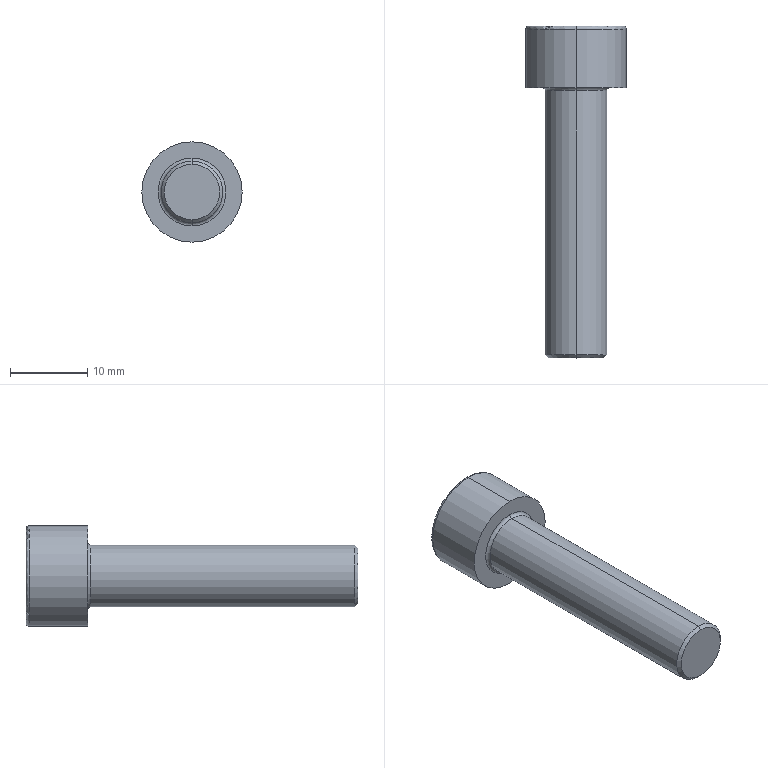Part | STEP file | 1 solid | 20 faces | box 13 x 43 x 13 mm | volume 2694 mm3 | plane 10 | torus 4 | cylinder 4 | cone 2 | commonest cylinder face diameters 8 x2 13 x2
STEP:
#1=CARTESIAN_POINT('',(0.,-35.,-3.6));
#2=VERTEX_POINT('',#1);
#3=CARTESIAN_POINT('',(0.,-35.,3.6));
#4=VERTEX_POINT('',#3);
#5=CARTESIAN_POINT('',(0.,-35.,0.));
#6=DIRECTION('',(0.,-1.,0.));
#7=DIRECTION('',(0.,0.,-1.));
#8=AXIS2_PLACEMENT_3D('',#5,#6,#7);
#9=CIRCLE('',#8,3.6);
#10=EDGE_CURVE('',#2,#4,#9,.T.);
#11=ORIENTED_EDGE('',*,*,#10,.F.);
#12=CARTESIAN_POINT('',(0.,-34.6,-4.));
#13=VERTEX_POINT('',#12);
#14=CARTESIAN_POINT('',(0.,-35.,-3.6));
#15=DIRECTION('',(0.,0.7071,-0.7071));
#16=VECTOR('',#15,1000.);
#17=LINE('',#14,#16);
#18=EDGE_CURVE('',#2,#13,#17,.T.);
#19=ORIENTED_EDGE('',*,*,#18,.T.);
#20=CARTESIAN_POINT('',(0.,-34.6,4.));
#21=VERTEX_POINT('',#20);
#22=CARTESIAN_POINT('',(0.,-34.6,0.));
#23=DIRECTION('',(0.,1.,0.));
#24=DIRECTION('',(0.,0.,-1.));
#25=AXIS2_PLACEMENT_3D('',#22,#23,#24);
#26=CIRCLE('',#25,4.);
#27=EDGE_CURVE('',#21,#13,#26,.T.);
#28=ORIENTED_EDGE('',*,*,#27,.F.);
#29=CARTESIAN_POINT('',(0.,-35.,3.6));
#30=DIRECTION('',(0.,0.7071,0.7071));
#31=VECTOR('',#30,1000.);
#32=LINE('',#29,#31);
#33=EDGE_CURVE('',#4,#21,#32,.T.);
#34=ORIENTED_EDGE('',*,*,#33,.F.);
#35=EDGE_LOOP('',(#11,#19,#28,#34));
#36=FACE_OUTER_BOUND('',#35,.T.);
#37=CARTESIAN_POINT('',(0.,-35.,0.));
#38=DIRECTION('',(0.,1.,0.));
#39=DIRECTION('',(0.,0.,1.));
#40=AXIS2_PLACEMENT_3D('',#37,#38,#39);
#41=CONICAL_SURFACE('',#40,3.6,0.7854);
#42=ADVANCED_FACE('',(#36),#41,.T.);
#43=CARTESIAN_POINT('',(0.,7.6,-6.5));
#44=VERTEX_POINT('',#43);
#45=CARTESIAN_POINT('',(0.,7.6,6.5));
#46=VERTEX_POINT('',#45);
#47=CARTESIAN_POINT('',(0.,7.6,0.));
#48=DIRECTION('',(0.,-1.,0.));
#49=DIRECTION('',(0.,0.,1.));
#50=AXIS2_PLACEMENT_3D('',#47,#48,#49);
#51=CIRCLE('',#50,6.5);
#52=EDGE_CURVE('',#44,#46,#51,.T.);
#53=ORIENTED_EDGE('',*,*,#52,.F.);
#54=CARTESIAN_POINT('',(0.,8.,-6.1));
#55=VERTEX_POINT('',#54);
#56=CARTESIAN_POINT('',(0.,7.6,-6.1));
#57=DIRECTION('',(1.,0.,0.));
#58=DIRECTION('',(0.,0.,-1.));
#59=AXIS2_PLACEMENT_3D('',#56,#57,#58);
#60=CIRCLE('',#59,0.4);
#61=EDGE_CURVE('',#44,#55,#60,.T.);
#62=ORIENTED_EDGE('',*,*,#61,.T.);
#63=CARTESIAN_POINT('',(0.,8.,6.1));
#64=VERTEX_POINT('',#63);
#65=CARTESIAN_POINT('',(0.,8.,0.));
#66=DIRECTION('',(0.,1.,0.));
#67=DIRECTION('',(0.,0.,1.));
#68=AXIS2_PLACEMENT_3D('',#65,#66,#67);
#69=CIRCLE('',#68,6.1);
#70=EDGE_CURVE('',#64,#55,#69,.T.);
#71=ORIENTED_EDGE('',*,*,#70,.F.);
#72=CARTESIAN_POINT('',(0.,7.6,6.1));
#73=DIRECTION('',(-1.,0.,0.));
#74=DIRECTION('',(0.,0.,1.));
#75=AXIS2_PLACEMENT_3D('',#72,#73,#74);
#76=CIRCLE('',#75,0.4);
#77=EDGE_CURVE('',#46,#64,#76,.T.);
#78=ORIENTED_EDGE('',*,*,#77,.F.);
#79=EDGE_LOOP('',(#53,#62,#71,#78));
#80=FACE_OUTER_BOUND('',#79,.T.);
#81=CARTESIAN_POINT('',(0.,7.6,0.));
#82=DIRECTION('',(0.,1.,0.));
#83=DIRECTION('',(0.,0.,1.));
#84=AXIS2_PLACEMENT_3D('',#81,#82,#83);
#85=TOROIDAL_SURFACE('',#84,6.1,0.4);
#86=ADVANCED_FACE('',(#80),#85,.T.);
#87=CARTESIAN_POINT('',(0.,-0.4,4.));
#88=VERTEX_POINT('',#87);
#89=CARTESIAN_POINT('',(0.,-0.4,-4.));
#90=VERTEX_POINT('',#89);
#91=CARTESIAN_POINT('',(0.,-0.4,0.));
#92=DIRECTION('',(0.,-1.,0.));
#93=DIRECTION('',(0.,0.,-1.));
#94=AXIS2_PLACEMENT_3D('',#91,#92,#93);
#95=CIRCLE('',#94,4.);
#96=EDGE_CURVE('',#88,#90,#95,.T.);
#97=ORIENTED_EDGE('',*,*,#96,.F.);
#98=CARTESIAN_POINT('',(0.,0.,4.4));
#99=VERTEX_POINT('',#98);
#100=CARTESIAN_POINT('',(0.,-0.4,4.4));
#101=DIRECTION('',(1.,0.,0.));
#102=DIRECTION('',(0.,0.,-1.));
#103=AXIS2_PLACEMENT_3D('',#100,#101,#102);
#104=CIRCLE('',#103,0.4);
#105=EDGE_CURVE('',#88,#99,#104,.T.);
#106=ORIENTED_EDGE('',*,*,#105,.T.);
#107=CARTESIAN_POINT('',(0.,0.,-4.4));
#108=VERTEX_POINT('',#107);
#109=CARTESIAN_POINT('',(0.,0.,0.));
#110=DIRECTION('',(0.,1.,0.));
#111=DIRECTION('',(0.,0.,-1.));
#112=AXIS2_PLACEMENT_3D('',#109,#110,#111);
#113=CIRCLE('',#112,4.4);
#114=EDGE_CURVE('',#108,#99,#113,.T.);
#115=ORIENTED_EDGE('',*,*,#114,.F.);
#116=CARTESIAN_POINT('',(0.,-0.4,-4.4));
#117=DIRECTION('',(-1.,0.,0.));
#118=DIRECTION('',(0.,0.,1.));
#119=AXIS2_PLACEMENT_3D('',#116,#117,#118);
#120=CIRCLE('',#119,0.4);
#121=EDGE_CURVE('',#90,#108,#120,.T.);
#122=ORIENTED_EDGE('',*,*,#121,.F.);
#123=EDGE_LOOP('',(#97,#106,#115,#122));
#124=FACE_OUTER_BOUND('',#123,.T.);
#125=CARTESIAN_POINT('',(0.,-0.4,0.));
#126=DIRECTION('',(0.,-1.,0.));
#127=DIRECTION('',(0.,0.,-1.));
#128=AXIS2_PLACEMENT_3D('',#125,#126,#127);
#129=TOROIDAL_SURFACE('',#128,4.4,0.4);
#130=ADVANCED_FACE('',(#124),#129,.F.);
#131=CARTESIAN_POINT('',(0.,-0.4,0.));
#132=DIRECTION('',(0.,-1.,0.));
#133=DIRECTION('',(0.,0.,-1.));
#134=AXIS2_PLACEMENT_3D('',#131,#132,#133);
#135=CIRCLE('',#134,4.);
#136=EDGE_CURVE('',#90,#88,#135,.T.);
#137=ORIENTED_EDGE('',*,*,#136,.T.);
#138=CARTESIAN_POINT('',(0.,0.,4.));
#139=DIRECTION('',(0.,-1.,0.));
#140=VECTOR('',#139,1000.);
#141=LINE('',#138,#140);
#142=EDGE_CURVE('',#88,#21,#141,.T.);
#143=ORIENTED_EDGE('',*,*,#142,.T.);
#144=ORIENTED_EDGE('',*,*,#27,.T.);
#145=CARTESIAN_POINT('',(0.,0.,-4.));
#146=DIRECTION('',(0.,-1.,0.));
#147=VECTOR('',#146,1000.);
#148=LINE('',#145,#147);
#149=EDGE_CURVE('',#90,#13,#148,.T.);
#150=ORIENTED_EDGE('',*,*,#149,.F.);
#151=EDGE_LOOP('',(#137,#143,#144,#150));
#152=FACE_OUTER_BOUND('',#151,.T.);
#153=CARTESIAN_POINT('',(0.,0.,0.));
#154=DIRECTION('',(0.,-1.,0.));
#155=DIRECTION('',(0.,0.,-1.));
#156=AXIS2_PLACEMENT_3D('',#153,#154,#155);
#157=CYLINDRICAL_SURFACE('',#156,4.);
#158=ADVANCED_FACE('',(#152),#157,.T.);
#159=ORIENTED_EDGE('',*,*,#52,.T.);
#160=CARTESIAN_POINT('',(0.,0.,6.5));
#161=VERTEX_POINT('',#160);
#162=CARTESIAN_POINT('',(0.,0.,6.5));
#163=DIRECTION('',(0.,-1.,0.));
#164=VECTOR('',#163,1000.);
#165=LINE('',#162,#164);
#166=EDGE_CURVE('',#46,#161,#165,.T.);
#167=ORIENTED_EDGE('',*,*,#166,.T.);
#168=CARTESIAN_POINT('',(0.,0.,-6.5));
#169=VERTEX_POINT('',#168);
#170=CARTESIAN_POINT('',(0.,0.,0.));
#171=DIRECTION('',(0.,-1.,0.));
#172=DIRECTION('',(0.,0.,-1.));
#173=AXIS2_PLACEMENT_3D('',#170,#171,#172);
#174=CIRCLE('',#173,6.5);
#175=EDGE_CURVE('',#169,#161,#174,.T.);
#176=ORIENTED_EDGE('',*,*,#175,.F.);
#177=CARTESIAN_POINT('',(0.,0.,-6.5));
#178=DIRECTION('',(0.,-1.,0.));
#179=VECTOR('',#178,1000.);
#180=LINE('',#177,#179);
#181=EDGE_CURVE('',#44,#169,#180,.T.);
#182=ORIENTED_EDGE('',*,*,#181,.F.);
#183=EDGE_LOOP('',(#159,#167,#176,#182));
#184=FACE_OUTER_BOUND('',#183,.T.);
#185=CARTESIAN_POINT('',(0.,0.,0.));
#186=DIRECTION('',(0.,-1.,0.));
#187=DIRECTION('',(0.,0.,-1.));
#188=AXIS2_PLACEMENT_3D('',#185,#186,#187);
#189=CYLINDRICAL_SURFACE('',#188,6.5);
#190=ADVANCED_FACE('',(#184),#189,.T.);
#191=ORIENTED_EDGE('',*,*,#70,.T.);
#192=CARTESIAN_POINT('',(0.,8.,0.));
#193=DIRECTION('',(0.,1.,0.));
#194=DIRECTION('',(0.,0.,1.));
#195=AXIS2_PLACEMENT_3D('',#192,#193,#194);
#196=CIRCLE('',#195,6.1);
#197=EDGE_CURVE('',#55,#64,#196,.T.);
#198=ORIENTED_EDGE('',*,*,#197,.T.);
#199=EDGE_LOOP('',(#191,#198));
#200=FACE_OUTER_BOUND('',#199,.T.);
#201=CARTESIAN_POINT('',(0.,8.,-3.464));
#202=VERTEX_POINT('',#201);
#203=CARTESIAN_POINT('',(-3.,8.,-1.732));
#204=VERTEX_POINT('',#203);
#205=CARTESIAN_POINT('',(0.,8.,-3.464));
#206=DIRECTION('',(-0.866,0.,0.5));
#207=VECTOR('',#206,1000.);
#208=LINE('',#205,#207);
#209=EDGE_CURVE('',#202,#204,#208,.T.);
#210=ORIENTED_EDGE('',*,*,#209,.F.);
#211=CARTESIAN_POINT('',(3.,8.,-1.732));
#212=VERTEX_POINT('',#211);
#213=CARTESIAN_POINT('',(3.,8.,-1.732));
#214=DIRECTION('',(-0.866,0.,-0.5));
#215=VECTOR('',#214,1000.);
#216=LINE('',#213,#215);
#217=EDGE_CURVE('',#212,#202,#216,.T.);
#218=ORIENTED_EDGE('',*,*,#217,.F.);
#219=CARTESIAN_POINT('',(3.,8.,1.732));
#220=VERTEX_POINT('',#219);
#221=CARTESIAN_POINT('',(3.,8.,1.732));
#222=DIRECTION('',(0.,0.,-1.));
#223=VECTOR('',#222,1000.);
#224=LINE('',#221,#223);
#225=EDGE_CURVE('',#220,#212,#224,.T.);
#226=ORIENTED_EDGE('',*,*,#225,.F.);
#227=CARTESIAN_POINT('',(0.,8.,3.464));
#228=VERTEX_POINT('',#227);
#229=CARTESIAN_POINT('',(0.,8.,3.464));
#230=DIRECTION('',(0.866,0.,-0.5));
#231=VECTOR('',#230,1000.);
#232=LINE('',#229,#231);
#233=EDGE_CURVE('',#228,#220,#232,.T.);
#234=ORIENTED_EDGE('',*,*,#233,.F.);
#235=CARTESIAN_POINT('',(-3.,8.,1.732));
#236=VERTEX_POINT('',#235);
#237=CARTESIAN_POINT('',(-3.,8.,1.732));
#238=DIRECTION('',(0.866,0.,0.5));
#239=VECTOR('',#238,1000.);
#240=LINE('',#237,#239);
#241=EDGE_CURVE('',#236,#228,#240,.T.);
#242=ORIENTED_EDGE('',*,*,#241,.F.);
#243=CARTESIAN_POINT('',(-3.,8.,-1.732));
#244=DIRECTION('',(0.,0.,1.));
#245=VECTOR('',#244,1000.);
#246=LINE('',#243,#245);
#247=EDGE_CURVE('',#204,#236,#246,.T.);
#248=ORIENTED_EDGE('',*,*,#247,.F.);
#249=EDGE_LOOP('',(#210,#218,#226,#234,#242,#248));
#250=FACE_BOUND('',#249,.T.);
#251=CARTESIAN_POINT('',(0.,8.,0.));
#252=DIRECTION('',(0.,1.,0.));
#253=DIRECTION('',(0.,0.,1.));
#254=AXIS2_PLACEMENT_3D('',#251,#252,#253);
#255=PLANE('',#254);
#256=ADVANCED_FACE('',(#200,#250),#255,.T.);
#257=ORIENTED_EDGE('',*,*,#166,.F.);
#258=CARTESIAN_POINT('',(0.,7.6,0.));
#259=DIRECTION('',(0.,-1.,0.));
#260=DIRECTION('',(0.,0.,1.));
#261=AXIS2_PLACEMENT_3D('',#258,#259,#260);
#262=CIRCLE('',#261,6.5);
#263=EDGE_CURVE('',#46,#44,#262,.T.);
#264=ORIENTED_EDGE('',*,*,#263,.T.);
#265=ORIENTED_EDGE('',*,*,#181,.T.);
#266=CARTESIAN_POINT('',(0.,0.,0.));
#267=DIRECTION('',(0.,-1.,0.));
#268=DIRECTION('',(0.,0.,-1.));
#269=AXIS2_PLACEMENT_3D('',#266,#267,#268);
#270=CIRCLE('',#269,6.5);
#271=EDGE_CURVE('',#161,#169,#270,.T.);
#272=ORIENTED_EDGE('',*,*,#271,.F.);
#273=EDGE_LOOP('',(#257,#264,#265,#272));
#274=FACE_OUTER_BOUND('',#273,.T.);
#275=CARTESIAN_POINT('',(0.,0.,0.));
#276=DIRECTION('',(0.,-1.,0.));
#277=DIRECTION('',(0.,0.,-1.));
#278=AXIS2_PLACEMENT_3D('',#275,#276,#277);
#279=CYLINDRICAL_SURFACE('',#278,6.5);
#280=ADVANCED_FACE('',(#274),#279,.T.);
#281=ORIENTED_EDGE('',*,*,#114,.T.);
#282=CARTESIAN_POINT('',(0.,0.,0.));
#283=DIRECTION('',(0.,1.,0.));
#284=DIRECTION('',(0.,0.,-1.));
#285=AXIS2_PLACEMENT_3D('',#282,#283,#284);
#286=CIRCLE('',#285,4.4);
#287=EDGE_CURVE('',#99,#108,#286,.T.);
#288=ORIENTED_EDGE('',*,*,#287,.T.);
#289=EDGE_LOOP('',(#281,#288));
#290=FACE_BOUND('',#289,.T.);
#291=ORIENTED_EDGE('',*,*,#175,.T.);
#292=ORIENTED_EDGE('',*,*,#271,.T.);
#293=EDGE_LOOP('',(#291,#292));
#294=FACE_OUTER_BOUND('',#293,.T.);
#295=CARTESIAN_POINT('',(6.5,0.,0.));
#296=DIRECTION('',(0.,-1.,0.));
#297=DIRECTION('',(0.,0.,-1.));
#298=AXIS2_PLACEMENT_3D('',#295,#296,#297);
#299=PLANE('',#298);
#300=ADVANCED_FACE('',(#290,#294),#299,.T.);
#301=ORIENTED_EDGE('',*,*,#142,.F.);
#302=ORIENTED_EDGE('',*,*,#96,.T.);
#303=ORIENTED_EDGE('',*,*,#149,.T.);
#304=CARTESIAN_POINT('',(0.,-34.6,0.));
#305=DIRECTION('',(0.,1.,0.));
#306=DIRECTION('',(0.,0.,-1.));
#307=AXIS2_PLACEMENT_3D('',#304,#305,#306);
#308=CIRCLE('',#307,4.);
#309=EDGE_CURVE('',#13,#21,#308,.T.);
#310=ORIENTED_EDGE('',*,*,#309,.T.);
#311=EDGE_LOOP('',(#301,#302,#303,#310));
#312=FACE_OUTER_BOUND('',#311,.T.);
#313=CARTESIAN_POINT('',(0.,0.,0.));
#314=DIRECTION('',(0.,-1.,0.));
#315=DIRECTION('',(0.,0.,-1.));
#316=AXIS2_PLACEMENT_3D('',#313,#314,#315);
#317=CYLINDRICAL_SURFACE('',#316,4.);
#318=ADVANCED_FACE('',(#312),#317,.T.);
#319=CARTESIAN_POINT('',(0.,-35.,0.));
#320=DIRECTION('',(0.,-1.,0.));
#321=DIRECTION('',(0.,0.,-1.));
#322=AXIS2_PLACEMENT_3D('',#319,#320,#321);
#323=CIRCLE('',#322,3.6);
#324=EDGE_CURVE('',#4,#2,#323,.T.);
#325=ORIENTED_EDGE('',*,*,#324,.T.);
#326=ORIENTED_EDGE('',*,*,#10,.T.);
#327=EDGE_LOOP('',(#325,#326));
#328=FACE_OUTER_BOUND('',#327,.T.);
#329=CARTESIAN_POINT('',(4.,-35.,0.));
#330=DIRECTION('',(0.,-1.,0.));
#331=DIRECTION('',(0.,0.,-1.));
#332=AXIS2_PLACEMENT_3D('',#329,#330,#331);
#333=PLANE('',#332);
#334=ADVANCED_FACE('',(#328),#333,.T.);
#335=ORIENTED_EDGE('',*,*,#209,.T.);
#336=CARTESIAN_POINT('',(-3.,4.,-1.732));
#337=VERTEX_POINT('',#336);
#338=CARTESIAN_POINT('',(-3.,4.,-1.732));
#339=DIRECTION('',(0.,1.,0.));
#340=VECTOR('',#339,1000.);
#341=LINE('',#338,#340);
#342=EDGE_CURVE('',#337,#204,#341,.T.);
#343=ORIENTED_EDGE('',*,*,#342,.F.);
#344=CARTESIAN_POINT('',(0.,4.,-3.464));
#345=VERTEX_POINT('',#344);
#346=CARTESIAN_POINT('',(0.,4.,-3.464));
#347=DIRECTION('',(-0.866,0.,0.5));
#348=VECTOR('',#347,1000.);
#349=LINE('',#346,#348);
#350=EDGE_CURVE('',#345,#337,#349,.T.);
#351=ORIENTED_EDGE('',*,*,#350,.F.);
#352=CARTESIAN_POINT('',(0.,4.,-3.464));
#353=DIRECTION('',(0.,1.,0.));
#354=VECTOR('',#353,1000.);
#355=LINE('',#352,#354);
#356=EDGE_CURVE('',#345,#202,#355,.T.);
#357=ORIENTED_EDGE('',*,*,#356,.T.);
#358=EDGE_LOOP('',(#335,#343,#351,#357));
#359=FACE_OUTER_BOUND('',#358,.T.);
#360=CARTESIAN_POINT('',(0.,4.,-3.464));
#361=DIRECTION('',(-0.5,0.,-0.866));
#362=DIRECTION('',(-0.866,0.,0.5));
#363=AXIS2_PLACEMENT_3D('',#360,#361,#362);
#364=PLANE('',#363);
#365=ADVANCED_FACE('',(#359),#364,.F.);
#366=ORIENTED_EDGE('',*,*,#217,.T.);
#367=ORIENTED_EDGE('',*,*,#356,.F.);
#368=CARTESIAN_POINT('',(3.,4.,-1.732));
#369=VERTEX_POINT('',#368);
#370=CARTESIAN_POINT('',(3.,4.,-1.732));
#371=DIRECTION('',(-0.866,0.,-0.5));
#372=VECTOR('',#371,1000.);
#373=LINE('',#370,#372);
#374=EDGE_CURVE('',#369,#345,#373,.T.);
#375=ORIENTED_EDGE('',*,*,#374,.F.);
#376=CARTESIAN_POINT('',(3.,4.,-1.732));
#377=DIRECTION('',(0.,1.,0.));
#378=VECTOR('',#377,1000.);
#379=LINE('',#376,#378);
#380=EDGE_CURVE('',#369,#212,#379,.T.);
#381=ORIENTED_EDGE('',*,*,#380,.T.);
#382=EDGE_LOOP('',(#366,#367,#375,#381));
#383=FACE_OUTER_BOUND('',#382,.T.);
#384=CARTESIAN_POINT('',(3.,4.,-1.732));
#385=DIRECTION('',(0.5,0.,-0.866));
#386=DIRECTION('',(-0.866,0.,-0.5));
#387=AXIS2_PLACEMENT_3D('',#384,#385,#386);
#388=PLANE('',#387);
#389=ADVANCED_FACE('',(#383),#388,.F.);
#390=ORIENTED_EDGE('',*,*,#225,.T.);
#391=ORIENTED_EDGE('',*,*,#380,.F.);
#392=CARTESIAN_POINT('',(3.,4.,1.732));
#393=VERTEX_POINT('',#392);
#394=CARTESIAN_POINT('',(3.,4.,1.732));
#395=DIRECTION('',(0.,0.,-1.));
#396=VECTOR('',#395,1000.);
#397=LINE('',#394,#396);
#398=EDGE_CURVE('',#393,#369,#397,.T.);
#399=ORIENTED_EDGE('',*,*,#398,.F.);
#400=CARTESIAN_POINT('',(3.,4.,1.732));
#401=DIRECTION('',(0.,1.,0.));
#402=VECTOR('',#401,1000.);
#403=LINE('',#400,#402);
#404=EDGE_CURVE('',#393,#220,#403,.T.);
#405=ORIENTED_EDGE('',*,*,#404,.T.);
#406=EDGE_LOOP('',(#390,#391,#399,#405));
#407=FACE_OUTER_BOUND('',#406,.T.);
#408=CARTESIAN_POINT('',(3.,4.,1.732));
#409=DIRECTION('',(1.,0.,0.));
#410=DIRECTION('',(0.,0.,-1.));
#411=AXIS2_PLACEMENT_3D('',#408,#409,#410);
#412=PLANE('',#411);
#413=ADVANCED_FACE('',(#407),#412,.F.);
#414=ORIENTED_EDGE('',*,*,#233,.T.);
#415=ORIENTED_EDGE('',*,*,#404,.F.);
#416=CARTESIAN_POINT('',(0.,4.,3.464));
#417=VERTEX_POINT('',#416);
#418=CARTESIAN_POINT('',(0.,4.,3.464));
#419=DIRECTION('',(0.866,0.,-0.5));
#420=VECTOR('',#419,1000.);
#421=LINE('',#418,#420);
#422=EDGE_CURVE('',#417,#393,#421,.T.);
#423=ORIENTED_EDGE('',*,*,#422,.F.);
#424=CARTESIAN_POINT('',(0.,4.,3.464));
#425=DIRECTION('',(0.,1.,0.));
#426=VECTOR('',#425,1000.);
#427=LINE('',#424,#426);
#428=EDGE_CURVE('',#417,#228,#427,.T.);
#429=ORIENTED_EDGE('',*,*,#428,.T.);
#430=EDGE_LOOP('',(#414,#415,#423,#429));
#431=FACE_OUTER_BOUND('',#430,.T.);
#432=CARTESIAN_POINT('',(0.,4.,3.464));
#433=DIRECTION('',(0.5,0.,0.866));
#434=DIRECTION('',(0.866,0.,-0.5));
#435=AXIS2_PLACEMENT_3D('',#432,#433,#434);
#436=PLANE('',#435);
#437=ADVANCED_FACE('',(#431),#436,.F.);
#438=ORIENTED_EDGE('',*,*,#241,.T.);
#439=ORIENTED_EDGE('',*,*,#428,.F.);
#440=CARTESIAN_POINT('',(-3.,4.,1.732));
#441=VERTEX_POINT('',#440);
#442=CARTESIAN_POINT('',(-3.,4.,1.732));
#443=DIRECTION('',(0.866,0.,0.5));
#444=VECTOR('',#443,1000.);
#445=LINE('',#442,#444);
#446=EDGE_CURVE('',#441,#417,#445,.T.);
#447=ORIENTED_EDGE('',*,*,#446,.F.);
#448=CARTESIAN_POINT('',(-3.,4.,1.732));
#449=DIRECTION('',(0.,1.,0.));
#450=VECTOR('',#449,1000.);
#451=LINE('',#448,#450);
#452=EDGE_CURVE('',#441,#236,#451,.T.);
#453=ORIENTED_EDGE('',*,*,#452,.T.);
#454=EDGE_LOOP('',(#438,#439,#447,#453));
#455=FACE_OUTER_BOUND('',#454,.T.);
#456=CARTESIAN_POINT('',(-3.,4.,1.732));
#457=DIRECTION('',(-0.5,0.,0.866));
#458=DIRECTION('',(0.866,0.,0.5));
#459=AXIS2_PLACEMENT_3D('',#456,#457,#458);
#460=PLANE('',#459);
#461=ADVANCED_FACE('',(#455),#460,.F.);
#462=ORIENTED_EDGE('',*,*,#247,.T.);
#463=ORIENTED_EDGE('',*,*,#452,.F.);
#464=CARTESIAN_POINT('',(-3.,4.,-1.732));
#465=DIRECTION('',(0.,0.,1.));
#466=VECTOR('',#465,1000.);
#467=LINE('',#464,#466);
#468=EDGE_CURVE('',#337,#441,#467,.T.);
#469=ORIENTED_EDGE('',*,*,#468,.F.);
#470=ORIENTED_EDGE('',*,*,#342,.T.);
#471=EDGE_LOOP('',(#462,#463,#469,#470));
#472=FACE_OUTER_BOUND('',#471,.T.);
#473=CARTESIAN_POINT('',(-3.,4.,-1.732));
#474=DIRECTION('',(-1.,0.,0.));
#475=DIRECTION('',(0.,0.,1.));
#476=AXIS2_PLACEMENT_3D('',#473,#474,#475);
#477=PLANE('',#476);
#478=ADVANCED_FACE('',(#472),#477,.F.);
#479=ORIENTED_EDGE('',*,*,#350,.T.);
#480=ORIENTED_EDGE('',*,*,#468,.T.);
#481=ORIENTED_EDGE('',*,*,#446,.T.);
#482=ORIENTED_EDGE('',*,*,#422,.T.);
#483=ORIENTED_EDGE('',*,*,#398,.T.);
#484=ORIENTED_EDGE('',*,*,#374,.T.);
#485=EDGE_LOOP('',(#479,#480,#481,#482,#483,#484));
#486=FACE_OUTER_BOUND('',#485,.T.);
#487=CARTESIAN_POINT('',(0.,4.,0.));
#488=DIRECTION('',(0.,1.,0.));
#489=DIRECTION('',(0.,0.,1.));
#490=AXIS2_PLACEMENT_3D('',#487,#488,#489);
#491=PLANE('',#490);
#492=ADVANCED_FACE('',(#486),#491,.T.);
#493=ORIENTED_EDGE('',*,*,#105,.F.);
#494=ORIENTED_EDGE('',*,*,#136,.F.);
#495=ORIENTED_EDGE('',*,*,#121,.T.);
#496=ORIENTED_EDGE('',*,*,#287,.F.);
#497=EDGE_LOOP('',(#493,#494,#495,#496));
#498=FACE_OUTER_BOUND('',#497,.T.);
#499=CARTESIAN_POINT('',(0.,-0.4,0.));
#500=DIRECTION('',(0.,-1.,0.));
#501=DIRECTION('',(0.,0.,-1.));
#502=AXIS2_PLACEMENT_3D('',#499,#500,#501);
#503=TOROIDAL_SURFACE('',#502,4.4,0.4);
#504=ADVANCED_FACE('',(#498),#503,.F.);
#505=ORIENTED_EDGE('',*,*,#61,.F.);
#506=ORIENTED_EDGE('',*,*,#263,.F.);
#507=ORIENTED_EDGE('',*,*,#77,.T.);
#508=ORIENTED_EDGE('',*,*,#197,.F.);
#509=EDGE_LOOP('',(#505,#506,#507,#508));
#510=FACE_OUTER_BOUND('',#509,.T.);
#511=CARTESIAN_POINT('',(0.,7.6,0.));
#512=DIRECTION('',(0.,1.,0.));
#513=DIRECTION('',(0.,0.,1.));
#514=AXIS2_PLACEMENT_3D('',#511,#512,#513);
#515=TOROIDAL_SURFACE('',#514,6.1,0.4);
#516=ADVANCED_FACE('',(#510),#515,.T.);
#517=ORIENTED_EDGE('',*,*,#18,.F.);
#518=ORIENTED_EDGE('',*,*,#324,.F.);
#519=ORIENTED_EDGE('',*,*,#33,.T.);
#520=ORIENTED_EDGE('',*,*,#309,.F.);
#521=EDGE_LOOP('',(#517,#518,#519,#520));
#522=FACE_OUTER_BOUND('',#521,.T.);
#523=CARTESIAN_POINT('',(0.,-35.,0.));
#524=DIRECTION('',(0.,1.,0.));
#525=DIRECTION('',(0.,0.,1.));
#526=AXIS2_PLACEMENT_3D('',#523,#524,#525);
#527=CONICAL_SURFACE('',#526,3.6,0.7854);
#528=ADVANCED_FACE('',(#522),#527,.T.);
#529=CLOSED_SHELL('',(#42,#86,#130,#158,#190,#256,#280,#300,#318,#334,#365,#389,#413,#437,#461,#478,#492,#504,#516,#528));
#530=MANIFOLD_SOLID_BREP('',#529);
#531=CARTESIAN_POINT('',(0.,0.,0.));
#532=DIRECTION('',(0.,0.,1.));
#533=DIRECTION('',(1.,0.,0.));
#534=AXIS2_PLACEMENT_3D('',#531,#532,#533);
#535=(LENGTH_UNIT()NAMED_UNIT(*)SI_UNIT(.MILLI.,.METRE.));
#536=UNCERTAINTY_MEASURE_WITH_UNIT(LENGTH_MEASURE(0.00001),#535,'','');
#537=(NAMED_UNIT(*)PLANE_ANGLE_UNIT()SI_UNIT($,.RADIAN.));
#538=(NAMED_UNIT(*)SI_UNIT($,.STERADIAN.)SOLID_ANGLE_UNIT());
#539=(GEOMETRIC_REPRESENTATION_CONTEXT(3)GLOBAL_UNCERTAINTY_ASSIGNED_CONTEXT((#536))GLOBAL_UNIT_ASSIGNED_CONTEXT((#535,#537,#538))REPRESENTATION_CONTEXT('',''));
#540=ADVANCED_BREP_SHAPE_REPRESENTATION('',(#530,#534),#539);